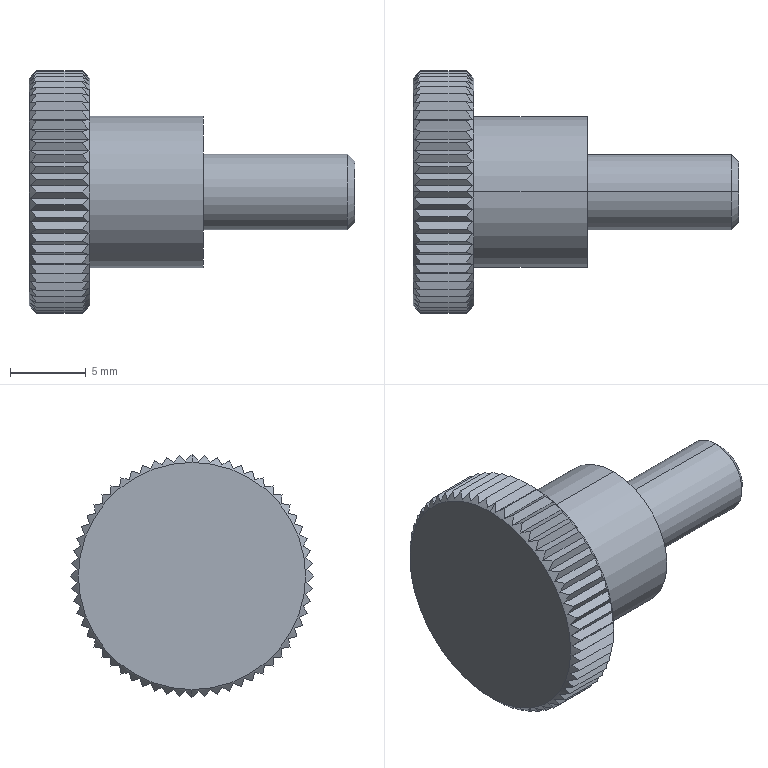Part | SolidWorks | features MBimport 1 | 1 solid | 134 faces | box 21.5 x 16 x 16 mm | volume 1542 mm3 | plane 124 | cone 6 | cylinder 4 | commonest cylinder face diameters 5 x2 10 x2